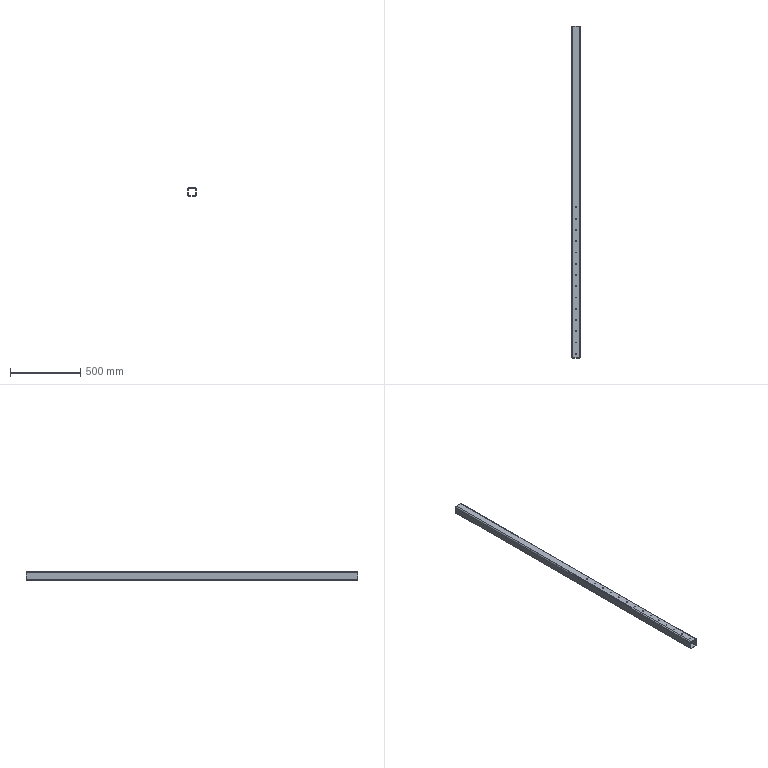Part | SolidWorks | features BaseBody 1 | 1 solid | 46 faces | box 60 x 2360 x 60 mm | volume 2015286 mm3 | cylinder 36 | plane 10 | commonest cylinder face diameters 6.8 x28 8 x4 16 x4